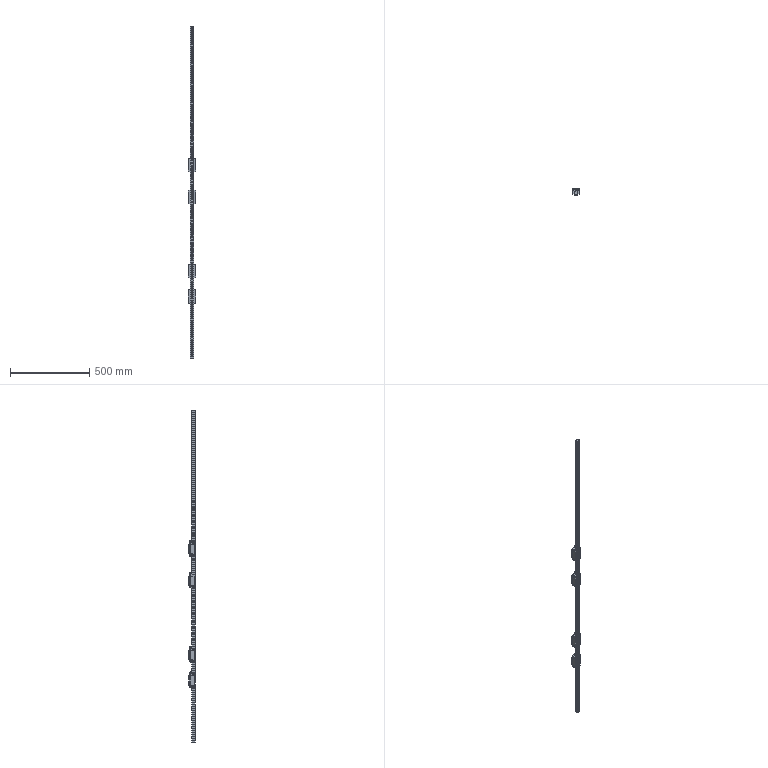Part | NX | features BREP 8 | 29 solids | 2603 faces | box 48 x 40 x 2100 mm | volume 1280258 mm3 | plane 1795 | cylinder 692 | cone 64 | torus 28 | sphere 16 | spline 8 | commonest cylinder face diameters 4.6 x84 7 x70 11 x70 0.207 x68 0.24 x68 6 x48